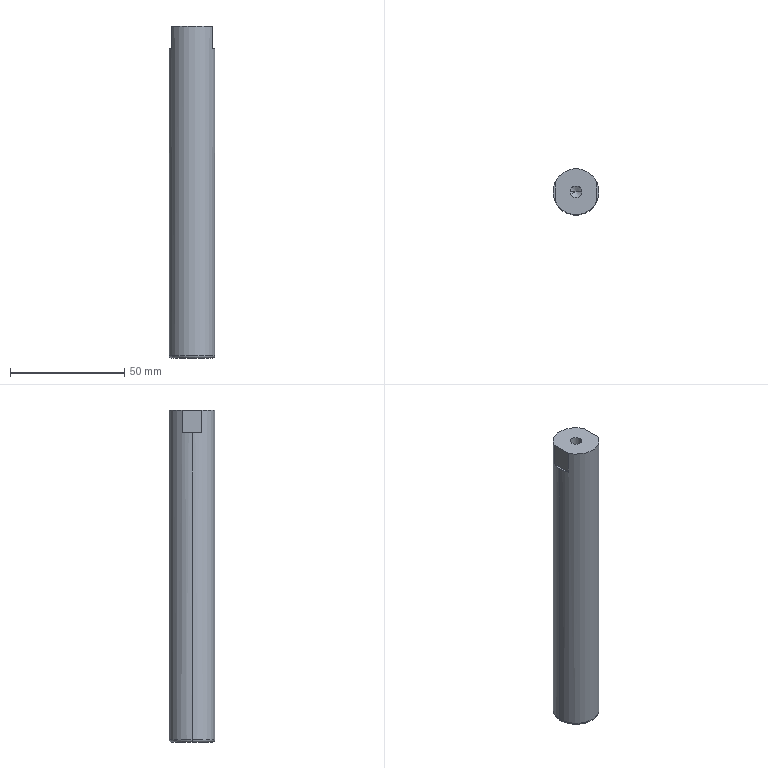Part | STEP file | 1 solid | 14 faces | box 20 x 20 x 145 mm | volume 45098 mm3 | plane 6 | cylinder 4 | torus 2 | cone 2 | commonest cylinder face diameters 5 x2 20 x2
STEP:
#1=CARTESIAN_POINT('',(0.,0.,0.));
#2=DIRECTION('',(0.,0.,1.));
#3=DIRECTION('',(1.,0.,0.));
#4=AXIS2_PLACEMENT_3D('',#1,#2,#3);
#5=CARTESIAN_POINT('',(-9.,0.,-72.5));
#6=VERTEX_POINT('',#5);
#7=CARTESIAN_POINT('',(9.,0.,-72.5));
#8=VERTEX_POINT('',#7);
#9=CARTESIAN_POINT('',(0.,0.,-72.5));
#10=DIRECTION('',(0.,0.,-1.));
#11=DIRECTION('',(1.,0.,0.));
#12=AXIS2_PLACEMENT_3D('',#9,#10,#11);
#13=CIRCLE('',#12,9.);
#14=CARTESIAN_POINT('',(0.,0.,-71.5));
#15=DIRECTION('',(0.,0.,1.));
#16=DIRECTION('',(1.,0.,0.));
#17=AXIS2_PLACEMENT_3D('',#14,#15,#16);
#18=TOROIDAL_SURFACE('',#17,9.,1.);
#19=CARTESIAN_POINT('',(6.283,4.712));
#20=DIRECTION('',(-1.,0.));
#21=VECTOR('',#20,1.);
#22=LINE('',#19,#21);
#23=(GEOMETRIC_REPRESENTATION_CONTEXT(2)PARAMETRIC_REPRESENTATION_CONTEXT()REPRESENTATION_CONTEXT('',''));
#24=DEFINITIONAL_REPRESENTATION('',(#22),#23);
#25=PCURVE('',#18,#24);
#26=CARTESIAN_POINT('',(0.,0.,-72.5));
#27=DIRECTION('',(0.,0.,1.));
#28=DIRECTION('',(1.,0.,0.));
#29=AXIS2_PLACEMENT_3D('',#26,#27,#28);
#30=PLANE('',#29);
#31=CARTESIAN_POINT('',(9.,0.));
#32=CARTESIAN_POINT('',(9.,-15.588));
#33=CARTESIAN_POINT('',(-4.5,-7.794));
#34=CARTESIAN_POINT('',(-18.,0.));
#35=CARTESIAN_POINT('',(-4.5,7.794));
#36=CARTESIAN_POINT('',(9.,15.588));
#37=CARTESIAN_POINT('',(9.,0.));
#38=(BOUNDED_CURVE()B_SPLINE_CURVE(2,(#31,#32,#33,#34,#35,#36,#37),.UNSPECIFIED.,.T.,.F.)B_SPLINE_CURVE_WITH_KNOTS((1,2,2,2,2,1),(-2.094,0.,2.094,4.189,6.283,8.378),.UNSPECIFIED.)CURVE()GEOMETRIC_REPRESENTATION_ITEM()RATIONAL_B_SPLINE_CURVE((1.,0.5,1.,0.5,1.,0.5,1.))REPRESENTATION_ITEM(''));
#39=(GEOMETRIC_REPRESENTATION_CONTEXT(2)PARAMETRIC_REPRESENTATION_CONTEXT()REPRESENTATION_CONTEXT('',''));
#40=DEFINITIONAL_REPRESENTATION('',(#38),#39);
#41=PCURVE('',#30,#40);
#42=SURFACE_CURVE('',#13,(#25,#41),.PCURVE_S1.);
#43=EDGE_CURVE('',#6,#8,#42,.T.);
#44=ORIENTED_EDGE('',*,*,#43,.F.);
#45=CARTESIAN_POINT('',(-10.,0.,-71.5));
#46=VERTEX_POINT('',#45);
#47=CARTESIAN_POINT('',(-9.,0.,-71.5));
#48=DIRECTION('',(0.,1.,0.));
#49=DIRECTION('',(-1.,0.,0.));
#50=AXIS2_PLACEMENT_3D('',#47,#48,#49);
#51=CIRCLE('',#50,1.);
#52=CARTESIAN_POINT('',(3.142,0.));
#53=DIRECTION('',(0.,1.));
#54=VECTOR('',#53,1.);
#55=LINE('',#52,#54);
#56=(GEOMETRIC_REPRESENTATION_CONTEXT(2)PARAMETRIC_REPRESENTATION_CONTEXT()REPRESENTATION_CONTEXT('',''));
#57=DEFINITIONAL_REPRESENTATION('',(#55),#56);
#58=PCURVE('',#18,#57);
#59=CARTESIAN_POINT('',(0.,0.,-71.5));
#60=DIRECTION('',(0.,0.,1.));
#61=DIRECTION('',(1.,0.,0.));
#62=AXIS2_PLACEMENT_3D('',#59,#60,#61);
#63=TOROIDAL_SURFACE('',#62,9.,1.);
#64=CARTESIAN_POINT('',(3.142,0.));
#65=DIRECTION('',(0.,1.));
#66=VECTOR('',#65,1.);
#67=LINE('',#64,#66);
#68=(GEOMETRIC_REPRESENTATION_CONTEXT(2)PARAMETRIC_REPRESENTATION_CONTEXT()REPRESENTATION_CONTEXT('',''));
#69=DEFINITIONAL_REPRESENTATION('',(#67),#68);
#70=PCURVE('',#63,#69);
#71=SURFACE_CURVE('',#51,(#58,#70),.PCURVE_S1.);
#72=EDGE_CURVE('',#6,#46,#71,.T.);
#73=ORIENTED_EDGE('',*,*,#72,.T.);
#74=CARTESIAN_POINT('',(10.,0.,-71.5));
#75=VERTEX_POINT('',#74);
#76=CARTESIAN_POINT('',(0.,0.,-71.5));
#77=DIRECTION('',(0.,0.,1.));
#78=DIRECTION('',(1.,0.,0.));
#79=AXIS2_PLACEMENT_3D('',#76,#77,#78);
#80=CIRCLE('',#79,10.);
#81=CARTESIAN_POINT('',(0.,6.283));
#82=DIRECTION('',(1.,0.));
#83=VECTOR('',#82,1.);
#84=LINE('',#81,#83);
#85=(GEOMETRIC_REPRESENTATION_CONTEXT(2)PARAMETRIC_REPRESENTATION_CONTEXT()REPRESENTATION_CONTEXT('',''));
#86=DEFINITIONAL_REPRESENTATION('',(#84),#85);
#87=PCURVE('',#18,#86);
#88=CARTESIAN_POINT('',(0.,0.,72.5));
#89=DIRECTION('',(0.,0.,-1.));
#90=DIRECTION('',(-1.,0.,0.));
#91=AXIS2_PLACEMENT_3D('',#88,#89,#90);
#92=CYLINDRICAL_SURFACE('',#91,10.);
#93=CARTESIAN_POINT('',(3.142,144.));
#94=DIRECTION('',(-1.,0.));
#95=VECTOR('',#94,1.);
#96=LINE('',#93,#95);
#97=(GEOMETRIC_REPRESENTATION_CONTEXT(2)PARAMETRIC_REPRESENTATION_CONTEXT()REPRESENTATION_CONTEXT('',''));
#98=DEFINITIONAL_REPRESENTATION('',(#96),#97);
#99=PCURVE('',#92,#98);
#100=SURFACE_CURVE('',#80,(#87,#99),.PCURVE_S1.);
#101=EDGE_CURVE('',#75,#46,#100,.T.);
#102=ORIENTED_EDGE('',*,*,#101,.F.);
#103=CARTESIAN_POINT('',(9.,0.,-71.5));
#104=DIRECTION('',(0.,-1.,0.));
#105=DIRECTION('',(0.,0.,-1.));
#106=AXIS2_PLACEMENT_3D('',#103,#104,#105);
#107=CIRCLE('',#106,1.);
#108=CARTESIAN_POINT('',(0.,4.712));
#109=DIRECTION('',(0.,1.));
#110=VECTOR('',#109,1.);
#111=LINE('',#108,#110);
#112=(GEOMETRIC_REPRESENTATION_CONTEXT(2)PARAMETRIC_REPRESENTATION_CONTEXT()REPRESENTATION_CONTEXT('',''));
#113=DEFINITIONAL_REPRESENTATION('',(#111),#112);
#114=PCURVE('',#18,#113);
#115=CARTESIAN_POINT('',(6.283,4.712));
#116=DIRECTION('',(0.,1.));
#117=VECTOR('',#116,1.);
#118=LINE('',#115,#117);
#119=(GEOMETRIC_REPRESENTATION_CONTEXT(2)PARAMETRIC_REPRESENTATION_CONTEXT()REPRESENTATION_CONTEXT('',''));
#120=DEFINITIONAL_REPRESENTATION('',(#118),#119);
#121=PCURVE('',#63,#120);
#122=SURFACE_CURVE('',#107,(#114,#121),.PCURVE_S1.);
#123=EDGE_CURVE('',#8,#75,#122,.T.);
#124=ORIENTED_EDGE('',*,*,#123,.F.);
#125=EDGE_LOOP('',(#44,#73,#102,#124));
#126=FACE_BOUND('',#125,.T.);
#127=ADVANCED_FACE('',(#126),#18,.T.);
#128=CARTESIAN_POINT('',(2.5,0.,56.5));
#129=VERTEX_POINT('',#128);
#130=CARTESIAN_POINT('',(2.5,0.,72.5));
#131=VERTEX_POINT('',#130);
#132=CARTESIAN_POINT('',(2.5,0.,72.5));
#133=DIRECTION('',(0.,0.,1.));
#134=VECTOR('',#133,1.);
#135=LINE('',#132,#134);
#136=CARTESIAN_POINT('',(0.,0.,72.5));
#137=DIRECTION('',(0.,0.,1.));
#138=DIRECTION('',(1.,0.,0.));
#139=AXIS2_PLACEMENT_3D('',#136,#137,#138);
#140=CYLINDRICAL_SURFACE('',#139,2.5);
#141=CARTESIAN_POINT('',(6.283,0.));
#142=DIRECTION('',(0.,1.));
#143=VECTOR('',#142,1.);
#144=LINE('',#141,#143);
#145=(GEOMETRIC_REPRESENTATION_CONTEXT(2)PARAMETRIC_REPRESENTATION_CONTEXT()REPRESENTATION_CONTEXT('',''));
#146=DEFINITIONAL_REPRESENTATION('',(#144),#145);
#147=PCURVE('',#140,#146);
#148=CARTESIAN_POINT('',(0.,0.,72.5));
#149=DIRECTION('',(0.,0.,1.));
#150=DIRECTION('',(1.,0.,0.));
#151=AXIS2_PLACEMENT_3D('',#148,#149,#150);
#152=CYLINDRICAL_SURFACE('',#151,2.5);
#153=CARTESIAN_POINT('',(0.,0.));
#154=DIRECTION('',(0.,1.));
#155=VECTOR('',#154,1.);
#156=LINE('',#153,#155);
#157=(GEOMETRIC_REPRESENTATION_CONTEXT(2)PARAMETRIC_REPRESENTATION_CONTEXT()REPRESENTATION_CONTEXT('',''));
#158=DEFINITIONAL_REPRESENTATION('',(#156),#157);
#159=PCURVE('',#152,#158);
#160=SURFACE_CURVE('',#135,(#147,#159),.PCURVE_S1.);
#161=EDGE_CURVE('',#129,#131,#160,.T.);
#162=ORIENTED_EDGE('',*,*,#161,.T.);
#163=CARTESIAN_POINT('',(-2.5,0.,72.5));
#164=VERTEX_POINT('',#163);
#165=CARTESIAN_POINT('',(0.,0.,72.5));
#166=DIRECTION('',(0.,0.,1.));
#167=DIRECTION('',(1.,0.,0.));
#168=AXIS2_PLACEMENT_3D('',#165,#166,#167);
#169=CIRCLE('',#168,2.5);
#170=CARTESIAN_POINT('',(0.,0.));
#171=DIRECTION('',(1.,0.));
#172=VECTOR('',#171,1.);
#173=LINE('',#170,#172);
#174=(GEOMETRIC_REPRESENTATION_CONTEXT(2)PARAMETRIC_REPRESENTATION_CONTEXT()REPRESENTATION_CONTEXT('',''));
#175=DEFINITIONAL_REPRESENTATION('',(#173),#174);
#176=PCURVE('',#140,#175);
#177=CARTESIAN_POINT('',(0.,0.,72.5));
#178=DIRECTION('',(0.,0.,1.));
#179=DIRECTION('',(1.,0.,0.));
#180=AXIS2_PLACEMENT_3D('',#177,#178,#179);
#181=PLANE('',#180);
#182=CARTESIAN_POINT('',(0.,0.));
#183=DIRECTION('',(1.,0.));
#184=AXIS2_PLACEMENT_2D('',#182,#183);
#185=CIRCLE('',#184,2.5);
#186=(GEOMETRIC_REPRESENTATION_CONTEXT(2)PARAMETRIC_REPRESENTATION_CONTEXT()REPRESENTATION_CONTEXT('',''));
#187=DEFINITIONAL_REPRESENTATION('',(#185),#186);
#188=PCURVE('',#181,#187);
#189=SURFACE_CURVE('',#169,(#176,#188),.PCURVE_S1.);
#190=EDGE_CURVE('',#164,#131,#189,.T.);
#191=ORIENTED_EDGE('',*,*,#190,.F.);
#192=CARTESIAN_POINT('',(-2.5,0.,56.5));
#193=VERTEX_POINT('',#192);
#194=CARTESIAN_POINT('',(-2.5,0.,72.5));
#195=DIRECTION('',(0.,0.,1.));
#196=VECTOR('',#195,1.);
#197=LINE('',#194,#196);
#198=CARTESIAN_POINT('',(3.142,0.));
#199=DIRECTION('',(0.,1.));
#200=VECTOR('',#199,1.);
#201=LINE('',#198,#200);
#202=(GEOMETRIC_REPRESENTATION_CONTEXT(2)PARAMETRIC_REPRESENTATION_CONTEXT()REPRESENTATION_CONTEXT('',''));
#203=DEFINITIONAL_REPRESENTATION('',(#201),#202);
#204=PCURVE('',#140,#203);
#205=CARTESIAN_POINT('',(3.142,0.));
#206=DIRECTION('',(0.,1.));
#207=VECTOR('',#206,1.);
#208=LINE('',#205,#207);
#209=(GEOMETRIC_REPRESENTATION_CONTEXT(2)PARAMETRIC_REPRESENTATION_CONTEXT()REPRESENTATION_CONTEXT('',''));
#210=DEFINITIONAL_REPRESENTATION('',(#208),#209);
#211=PCURVE('',#152,#210);
#212=SURFACE_CURVE('',#197,(#204,#211),.PCURVE_S1.);
#213=EDGE_CURVE('',#193,#164,#212,.T.);
#214=ORIENTED_EDGE('',*,*,#213,.F.);
#215=CARTESIAN_POINT('',(0.,0.,56.5));
#216=DIRECTION('',(0.,0.,1.));
#217=DIRECTION('',(1.,0.,0.));
#218=AXIS2_PLACEMENT_3D('',#215,#216,#217);
#219=CIRCLE('',#218,2.5);
#220=CARTESIAN_POINT('',(0.,-16.));
#221=DIRECTION('',(1.,0.));
#222=VECTOR('',#221,1.);
#223=LINE('',#220,#222);
#224=(GEOMETRIC_REPRESENTATION_CONTEXT(2)PARAMETRIC_REPRESENTATION_CONTEXT()REPRESENTATION_CONTEXT('',''));
#225=DEFINITIONAL_REPRESENTATION('',(#223),#224);
#226=PCURVE('',#140,#225);
#227=CARTESIAN_POINT('',(0.,0.,56.5));
#228=DIRECTION('',(0.,0.,1.));
#229=DIRECTION('',(1.,0.,0.));
#230=AXIS2_PLACEMENT_3D('',#227,#228,#229);
#231=CONICAL_SURFACE('',#230,2.5,1.03);
#232=CARTESIAN_POINT('',(0.,0.));
#233=DIRECTION('',(1.,0.));
#234=VECTOR('',#233,1.);
#235=LINE('',#232,#234);
#236=(GEOMETRIC_REPRESENTATION_CONTEXT(2)PARAMETRIC_REPRESENTATION_CONTEXT()REPRESENTATION_CONTEXT('',''));
#237=DEFINITIONAL_REPRESENTATION('',(#235),#236);
#238=PCURVE('',#231,#237);
#239=SURFACE_CURVE('',#219,(#226,#238),.PCURVE_S1.);
#240=EDGE_CURVE('',#193,#129,#239,.T.);
#241=ORIENTED_EDGE('',*,*,#240,.T.);
#242=EDGE_LOOP('',(#162,#191,#214,#241));
#243=FACE_BOUND('',#242,.F.);
#244=ADVANCED_FACE('',(#243),#140,.F.);
#245=ORIENTED_EDGE('',*,*,#240,.F.);
#246=CARTESIAN_POINT('',(0.,0.,54.998));
#247=VERTEX_POINT('',#246);
#248=CARTESIAN_POINT('',(-2.5,0.,56.5));
#249=DIRECTION('',(-0.8572,0.,0.515));
#250=VECTOR('',#249,1.);
#251=LINE('',#248,#250);
#252=CARTESIAN_POINT('',(3.142,0.));
#253=DIRECTION('',(0.,1.));
#254=VECTOR('',#253,1.);
#255=LINE('',#252,#254);
#256=(GEOMETRIC_REPRESENTATION_CONTEXT(2)PARAMETRIC_REPRESENTATION_CONTEXT()REPRESENTATION_CONTEXT('',''));
#257=DEFINITIONAL_REPRESENTATION('',(#255),#256);
#258=PCURVE('',#231,#257);
#259=CARTESIAN_POINT('',(0.,0.,56.5));
#260=DIRECTION('',(0.,0.,1.));
#261=DIRECTION('',(1.,0.,0.));
#262=AXIS2_PLACEMENT_3D('',#259,#260,#261);
#263=CONICAL_SURFACE('',#262,2.5,1.03);
#264=CARTESIAN_POINT('',(3.142,0.));
#265=DIRECTION('',(0.,1.));
#266=VECTOR('',#265,1.);
#267=LINE('',#264,#266);
#268=(GEOMETRIC_REPRESENTATION_CONTEXT(2)PARAMETRIC_REPRESENTATION_CONTEXT()REPRESENTATION_CONTEXT('',''));
#269=DEFINITIONAL_REPRESENTATION('',(#267),#268);
#270=PCURVE('',#263,#269);
#271=SURFACE_CURVE('',#251,(#258,#270),.PCURVE_S1.);
#272=EDGE_CURVE('',#247,#193,#271,.T.);
#273=ORIENTED_EDGE('',*,*,#272,.F.);
#274=CARTESIAN_POINT('',(2.5,0.,56.5));
#275=DIRECTION('',(0.8572,0.,0.515));
#276=VECTOR('',#275,1.);
#277=LINE('',#274,#276);
#278=CARTESIAN_POINT('',(6.283,0.));
#279=DIRECTION('',(0.,1.));
#280=VECTOR('',#279,1.);
#281=LINE('',#278,#280);
#282=(GEOMETRIC_REPRESENTATION_CONTEXT(2)PARAMETRIC_REPRESENTATION_CONTEXT()REPRESENTATION_CONTEXT('',''));
#283=DEFINITIONAL_REPRESENTATION('',(#281),#282);
#284=PCURVE('',#231,#283);
#285=CARTESIAN_POINT('',(0.,0.));
#286=DIRECTION('',(0.,1.));
#287=VECTOR('',#286,1.);
#288=LINE('',#285,#287);
#289=(GEOMETRIC_REPRESENTATION_CONTEXT(2)PARAMETRIC_REPRESENTATION_CONTEXT()REPRESENTATION_CONTEXT('',''));
#290=DEFINITIONAL_REPRESENTATION('',(#288),#289);
#291=PCURVE('',#263,#290);
#292=SURFACE_CURVE('',#277,(#284,#291),.PCURVE_S1.);
#293=EDGE_CURVE('',#247,#129,#292,.T.);
#294=ORIENTED_EDGE('',*,*,#293,.T.);
#295=EDGE_LOOP('',(#245,#273,#294));
#296=FACE_BOUND('',#295,.F.);
#297=ADVANCED_FACE('',(#296),#231,.F.);
#298=CARTESIAN_POINT('',(10.,0.,62.5));
#299=VERTEX_POINT('',#298);
#300=CARTESIAN_POINT('',(9.,4.359,62.5));
#301=VERTEX_POINT('',#300);
#302=CARTESIAN_POINT('',(0.,0.,62.5));
#303=DIRECTION('',(0.,0.,1.));
#304=DIRECTION('',(1.,0.,0.));
#305=AXIS2_PLACEMENT_3D('',#302,#303,#304);
#306=CIRCLE('',#305,10.);
#307=CARTESIAN_POINT('',(3.142,10.));
#308=DIRECTION('',(-1.,0.));
#309=VECTOR('',#308,1.);
#310=LINE('',#307,#309);
#311=(GEOMETRIC_REPRESENTATION_CONTEXT(2)PARAMETRIC_REPRESENTATION_CONTEXT()REPRESENTATION_CONTEXT('',''));
#312=DEFINITIONAL_REPRESENTATION('',(#310),#311);
#313=PCURVE('',#92,#312);
#314=CARTESIAN_POINT('',(0.,0.,62.5));
#315=DIRECTION('',(0.,0.,1.));
#316=DIRECTION('',(1.,0.,0.));
#317=AXIS2_PLACEMENT_3D('',#314,#315,#316);
#318=PLANE('',#317);
#319=CARTESIAN_POINT('',(0.,0.));
#320=DIRECTION('',(1.,0.));
#321=AXIS2_PLACEMENT_2D('',#319,#320);
#322=CIRCLE('',#321,10.);
#323=(GEOMETRIC_REPRESENTATION_CONTEXT(2)PARAMETRIC_REPRESENTATION_CONTEXT()REPRESENTATION_CONTEXT('',''));
#324=DEFINITIONAL_REPRESENTATION('',(#322),#323);
#325=PCURVE('',#318,#324);
#326=SURFACE_CURVE('',#306,(#313,#325),.PCURVE_S1.);
#327=EDGE_CURVE('',#299,#301,#326,.T.);
#328=ORIENTED_EDGE('',*,*,#327,.F.);
#329=CARTESIAN_POINT('',(10.,0.,72.5));
#330=DIRECTION('',(0.,0.,-1.));
#331=VECTOR('',#330,1.);
#332=LINE('',#329,#331);
#333=CARTESIAN_POINT('',(3.142,0.));
#334=DIRECTION('',(0.,1.));
#335=VECTOR('',#334,1.);
#336=LINE('',#333,#335);
#337=(GEOMETRIC_REPRESENTATION_CONTEXT(2)PARAMETRIC_REPRESENTATION_CONTEXT()REPRESENTATION_CONTEXT('',''));
#338=DEFINITIONAL_REPRESENTATION('',(#336),#337);
#339=PCURVE('',#92,#338);
#340=CARTESIAN_POINT('',(0.,0.,72.5));
#341=DIRECTION('',(0.,0.,-1.));
#342=DIRECTION('',(-1.,0.,0.));
#343=AXIS2_PLACEMENT_3D('',#340,#341,#342);
#344=CYLINDRICAL_SURFACE('',#343,10.);
#345=CARTESIAN_POINT('',(3.142,0.));
#346=DIRECTION('',(0.,1.));
#347=VECTOR('',#346,1.);
#348=LINE('',#345,#347);
#349=(GEOMETRIC_REPRESENTATION_CONTEXT(2)PARAMETRIC_REPRESENTATION_CONTEXT()REPRESENTATION_CONTEXT('',''));
#350=DEFINITIONAL_REPRESENTATION('',(#348),#349);
#351=PCURVE('',#344,#350);
#352=SURFACE_CURVE('',#332,(#339,#351),.PCURVE_S1.);
#353=EDGE_CURVE('',#299,#75,#352,.T.);
#354=ORIENTED_EDGE('',*,*,#353,.T.);
#355=ORIENTED_EDGE('',*,*,#101,.T.);
#356=CARTESIAN_POINT('',(-10.,0.,62.5));
#357=VERTEX_POINT('',#356);
#358=CARTESIAN_POINT('',(-10.,0.,72.5));
#359=DIRECTION('',(0.,0.,-1.));
#360=VECTOR('',#359,1.);
#361=LINE('',#358,#360);
#362=CARTESIAN_POINT('',(0.,0.));
#363=DIRECTION('',(0.,1.));
#364=VECTOR('',#363,1.);
#365=LINE('',#362,#364);
#366=(GEOMETRIC_REPRESENTATION_CONTEXT(2)PARAMETRIC_REPRESENTATION_CONTEXT()REPRESENTATION_CONTEXT('',''));
#367=DEFINITIONAL_REPRESENTATION('',(#365),#366);
#368=PCURVE('',#92,#367);
#369=CARTESIAN_POINT('',(6.283,0.));
#370=DIRECTION('',(0.,1.));
#371=VECTOR('',#370,1.);
#372=LINE('',#369,#371);
#373=(GEOMETRIC_REPRESENTATION_CONTEXT(2)PARAMETRIC_REPRESENTATION_CONTEXT()REPRESENTATION_CONTEXT('',''));
#374=DEFINITIONAL_REPRESENTATION('',(#372),#373);
#375=PCURVE('',#344,#374);
#376=SURFACE_CURVE('',#361,(#368,#375),.PCURVE_S1.);
#377=EDGE_CURVE('',#357,#46,#376,.T.);
#378=ORIENTED_EDGE('',*,*,#377,.F.);
#379=CARTESIAN_POINT('',(-9.,4.359,62.5));
#380=VERTEX_POINT('',#379);
#381=CARTESIAN_POINT('',(0.,0.,62.5));
#382=DIRECTION('',(0.,0.,1.));
#383=DIRECTION('',(1.,0.,0.));
#384=AXIS2_PLACEMENT_3D('',#381,#382,#383);
#385=CIRCLE('',#384,10.);
#386=CARTESIAN_POINT('',(3.142,10.));
#387=DIRECTION('',(-1.,0.));
#388=VECTOR('',#387,1.);
#389=LINE('',#386,#388);
#390=(GEOMETRIC_REPRESENTATION_CONTEXT(2)PARAMETRIC_REPRESENTATION_CONTEXT()REPRESENTATION_CONTEXT('',''));
#391=DEFINITIONAL_REPRESENTATION('',(#389),#390);
#392=PCURVE('',#92,#391);
#393=CARTESIAN_POINT('',(0.,0.,62.5));
#394=DIRECTION('',(0.,0.,1.));
#395=DIRECTION('',(1.,0.,0.));
#396=AXIS2_PLACEMENT_3D('',#393,#394,#395);
#397=PLANE('',#396);
#398=CARTESIAN_POINT('',(0.,0.));
#399=DIRECTION('',(1.,0.));
#400=AXIS2_PLACEMENT_2D('',#398,#399);
#401=CIRCLE('',#400,10.);
#402=(GEOMETRIC_REPRESENTATION_CONTEXT(2)PARAMETRIC_REPRESENTATION_CONTEXT()REPRESENTATION_CONTEXT('',''));
#403=DEFINITIONAL_REPRESENTATION('',(#401),#402);
#404=PCURVE('',#397,#403);
#405=SURFACE_CURVE('',#385,(#392,#404),.PCURVE_S1.);
#406=EDGE_CURVE('',#380,#357,#405,.T.);
#407=ORIENTED_EDGE('',*,*,#406,.F.);
#408=CARTESIAN_POINT('',(-9.,4.359,72.5));
#409=VERTEX_POINT('',#408);
#410=CARTESIAN_POINT('',(-9.,4.359,72.5));
#411=DIRECTION('',(0.,0.,-1.));
#412=VECTOR('',#411,1.);
#413=LINE('',#410,#412);
#414=CARTESIAN_POINT('',(0.451,0.));
#415=DIRECTION('',(0.,1.));
#416=VECTOR('',#415,1.);
#417=LINE('',#414,#416);
#418=(GEOMETRIC_REPRESENTATION_CONTEXT(2)PARAMETRIC_REPRESENTATION_CONTEXT()REPRESENTATION_CONTEXT('',''));
#419=DEFINITIONAL_REPRESENTATION('',(#417),#418);
#420=PCURVE('',#92,#419);
#421=CARTESIAN_POINT('',(-9.,-11.827,62.5));
#422=DIRECTION('',(-1.,0.,0.));
#423=DIRECTION('',(0.,0.,1.));
#424=AXIS2_PLACEMENT_3D('',#421,#422,#423);
#425=PLANE('',#424);
#426=CARTESIAN_POINT('',(10.,16.185));
#427=DIRECTION('',(-1.,0.));
#428=VECTOR('',#427,1.);
#429=LINE('',#426,#428);
#430=(GEOMETRIC_REPRESENTATION_CONTEXT(2)PARAMETRIC_REPRESENTATION_CONTEXT()REPRESENTATION_CONTEXT('',''));
#431=DEFINITIONAL_REPRESENTATION('',(#429),#430);
#432=PCURVE('',#425,#431);
#433=SURFACE_CURVE('',#413,(#420,#432),.PCURVE_S1.);
#434=EDGE_CURVE('',#409,#380,#433,.T.);
#435=ORIENTED_EDGE('',*,*,#434,.F.);
#436=CARTESIAN_POINT('',(9.,4.359,72.5));
#437=VERTEX_POINT('',#436);
#438=CARTESIAN_POINT('',(0.,0.,72.5));
#439=DIRECTION('',(0.,0.,1.));
#440=DIRECTION('',(1.,0.,0.));
#441=AXIS2_PLACEMENT_3D('',#438,#439,#440);
#442=CIRCLE('',#441,10.);
#443=CARTESIAN_POINT('',(3.142,0.));
#444=DIRECTION('',(-1.,0.));
#445=VECTOR('',#444,1.);
#446=LINE('',#443,#445);
#447=(GEOMETRIC_REPRESENTATION_CONTEXT(2)PARAMETRIC_REPRESENTATION_CONTEXT()REPRESENTATION_CONTEXT('',''));
#448=DEFINITIONAL_REPRESENTATION('',(#446),#447);
#449=PCURVE('',#92,#448);
#450=CARTESIAN_POINT('',(0.,0.));
#451=DIRECTION('',(1.,0.));
#452=AXIS2_PLACEMENT_2D('',#450,#451);
#453=CIRCLE('',#452,10.);
#454=(GEOMETRIC_REPRESENTATION_CONTEXT(2)PARAMETRIC_REPRESENTATION_CONTEXT()REPRESENTATION_CONTEXT('',''));
#455=DEFINITIONAL_REPRESENTATION('',(#453),#454);
#456=PCURVE('',#181,#455);
#457=SURFACE_CURVE('',#442,(#449,#456),.PCURVE_S1.);
#458=EDGE_CURVE('',#437,#409,#457,.T.);
#459=ORIENTED_EDGE('',*,*,#458,.F.);
#460=CARTESIAN_POINT('',(9.,4.359,72.5));
#461=DIRECTION('',(0.,0.,1.));
#462=VECTOR('',#461,1.);
#463=LINE('',#460,#462);
#464=CARTESIAN_POINT('',(2.691,0.));
#465=DIRECTION('',(0.,-1.));
#466=VECTOR('',#465,1.);
#467=LINE('',#464,#466);
#468=(GEOMETRIC_REPRESENTATION_CONTEXT(2)PARAMETRIC_REPRESENTATION_CONTEXT()REPRESENTATION_CONTEXT('',''));
#469=DEFINITIONAL_REPRESENTATION('',(#467),#468);
#470=PCURVE('',#92,#469);
#471=CARTESIAN_POINT('',(9.,-11.827,62.5));
#472=DIRECTION('',(1.,0.,0.));
#473=DIRECTION('',(0.,0.,-1.));
#474=AXIS2_PLACEMENT_3D('',#471,#472,#473);
#475=PLANE('',#474);
#476=CARTESIAN_POINT('',(-10.,16.185));
#477=DIRECTION('',(-1.,0.));
#478=VECTOR('',#477,1.);
#479=LINE('',#476,#478);
#480=(GEOMETRIC_REPRESENTATION_CONTEXT(2)PARAMETRIC_REPRESENTATION_CONTEXT()REPRESENTATION_CONTEXT('',''));
#481=DEFINITIONAL_REPRESENTATION('',(#479),#480);
#482=PCURVE('',#475,#481);
#483=SURFACE_CURVE('',#463,(#470,#482),.PCURVE_S1.);
#484=EDGE_CURVE('',#301,#437,#483,.T.);
#485=ORIENTED_EDGE('',*,*,#484,.F.);
#486=EDGE_LOOP('',(#328,#354,#355,#378,#407,#435,#459,#485));
#487=FACE_BOUND('',#486,.T.);
#488=ADVANCED_FACE('',(#487),#92,.T.);
#489=ORIENTED_EDGE('',*,*,#353,.F.);
#490=CARTESIAN_POINT('',(9.,-4.359,62.5));
#491=VERTEX_POINT('',#490);
#492=CARTESIAN_POINT('',(0.,0.,62.5));
#493=DIRECTION('',(0.,0.,1.));
#494=DIRECTION('',(1.,0.,0.));
#495=AXIS2_PLACEMENT_3D('',#492,#493,#494);
#496=CIRCLE('',#495,10.);
#497=CARTESIAN_POINT('',(9.425,10.));
#498=DIRECTION('',(-1.,0.));
#499=VECTOR('',#498,1.);
#500=LINE('',#497,#499);
#501=(GEOMETRIC_REPRESENTATION_CONTEXT(2)PARAMETRIC_REPRESENTATION_CONTEXT()REPRESENTATION_CONTEXT('',''));
#502=DEFINITIONAL_REPRESENTATION('',(#500),#501);
#503=PCURVE('',#344,#502);
#504=CARTESIAN_POINT('',(0.,0.));
#505=DIRECTION('',(1.,0.));
#506=AXIS2_PLACEMENT_2D('',#504,#505);
#507=CIRCLE('',#506,10.);
#508=(GEOMETRIC_REPRESENTATION_CONTEXT(2)PARAMETRIC_REPRESENTATION_CONTEXT()REPRESENTATION_CONTEXT('',''));
#509=DEFINITIONAL_REPRESENTATION('',(#507),#508);
#510=PCURVE('',#318,#509);
#511=SURFACE_CURVE('',#496,(#503,#510),.PCURVE_S1.);
#512=EDGE_CURVE('',#491,#299,#511,.T.);
#513=ORIENTED_EDGE('',*,*,#512,.F.);
#514=CARTESIAN_POINT('',(9.,-4.359,72.5));
#515=VERTEX_POINT('',#514);
#516=CARTESIAN_POINT('',(9.,-4.359,72.5));
#517=DIRECTION('',(0.,0.,-1.));
#518=VECTOR('',#517,1.);
#519=LINE('',#516,#518);
#520=CARTESIAN_POINT('',(3.593,0.));
#521=DIRECTION('',(0.,1.));
#522=VECTOR('',#521,1.);
#523=LINE('',#520,#522);
#524=(GEOMETRIC_REPRESENTATION_CONTEXT(2)PARAMETRIC_REPRESENTATION_CONTEXT()REPRESENTATION_CONTEXT('',''));
#525=DEFINITIONAL_REPRESENTATION('',(#523),#524);
#526=PCURVE('',#344,#525);
#527=CARTESIAN_POINT('',(-10.,7.468));
#528=DIRECTION('',(1.,0.));
#529=VECTOR('',#528,1.);
#530=LINE('',#527,#529);
#531=(GEOMETRIC_REPRESENTATION_CONTEXT(2)PARAMETRIC_REPRESENTATION_CONTEXT()REPRESENTATION_CONTEXT('',''));
#532=DEFINITIONAL_REPRESENTATION('',(#530),#531);
#533=PCURVE('',#475,#532);
#534=SURFACE_CURVE('',#519,(#526,#533),.PCURVE_S1.);
#535=EDGE_CURVE('',#515,#491,#534,.T.);
#536=ORIENTED_EDGE('',*,*,#535,.F.);
#537=CARTESIAN_POINT('',(-9.,-4.359,72.5));
#538=VERTEX_POINT('',#537);
#539=CARTESIAN_POINT('',(0.,0.,72.5));
#540=DIRECTION('',(0.,0.,1.));
#541=DIRECTION('',(1.,0.,0.));
#542=AXIS2_PLACEMENT_3D('',#539,#540,#541);
#543=CIRCLE('',#542,10.);
#544=CARTESIAN_POINT('',(9.425,0.));
#545=DIRECTION('',(-1.,0.));
#546=VECTOR('',#545,1.);
#547=LINE('',#544,#546);
#548=(GEOMETRIC_REPRESENTATION_CONTEXT(2)PARAMETRIC_REPRESENTATION_CONTEXT()REPRESENTATION_CONTEXT('',''));
#549=DEFINITIONAL_REPRESENTATION('',(#547),#548);
#550=PCURVE('',#344,#549);
#551=CARTESIAN_POINT('',(0.,0.));
#552=DIRECTION('',(1.,0.));
#553=AXIS2_PLACEMENT_2D('',#551,#552);
#554=CIRCLE('',#553,10.);
#555=(GEOMETRIC_REPRESENTATION_CONTEXT(2)PARAMETRIC_REPRESENTATION_CONTEXT()REPRESENTATION_CONTEXT('',''));
#556=DEFINITIONAL_REPRESENTATION('',(#554),#555);
#557=PCURVE('',#181,#556);
#558=SURFACE_CURVE('',#543,(#550,#557),.PCURVE_S1.);
#559=EDGE_CURVE('',#538,#515,#558,.T.);
#560=ORIENTED_EDGE('',*,*,#559,.F.);
#561=CARTESIAN_POINT('',(-9.,-4.359,62.5));
#562=VERTEX_POINT('',#561);
#563=CARTESIAN_POINT('',(-9.,-4.359,72.5));
#564=DIRECTION('',(0.,0.,1.));
#565=VECTOR('',#564,1.);
#566=LINE('',#563,#565);
#567=CARTESIAN_POINT('',(5.832,0.));
#568=DIRECTION('',(0.,-1.));
#569=VECTOR('',#568,1.);
#570=LINE('',#567,#569);
#571=(GEOMETRIC_REPRESENTATION_CONTEXT(2)PARAMETRIC_REPRESENTATION_CONTEXT()REPRESENTATION_CONTEXT('',''));
#572=DEFINITIONAL_REPRESENTATION('',(#570),#571);
#573=PCURVE('',#344,#572);
#574=CARTESIAN_POINT('',(10.,7.468));
#575=DIRECTION('',(1.,0.));
#576=VECTOR('',#575,1.);
#577=LINE('',#574,#576);
#578=(GEOMETRIC_REPRESENTATION_CONTEXT(2)PARAMETRIC_REPRESENTATION_CONTEXT()REPRESENTATION_CONTEXT('',''));
#579=DEFINITIONAL_REPRESENTATION('',(#577),#578);
#580=PCURVE('',#425,#579);
#581=SURFACE_CURVE('',#566,(#573,#580),.PCURVE_S1.);
#582=EDGE_CURVE('',#562,#538,#581,.T.);
#583=ORIENTED_EDGE('',*,*,#582,.F.);
#584=CARTESIAN_POINT('',(0.,0.,62.5));
#585=DIRECTION('',(0.,0.,1.));
#586=DIRECTION('',(1.,0.,0.));
#587=AXIS2_PLACEMENT_3D('',#584,#585,#586);
#588=CIRCLE('',#587,10.);
#589=CARTESIAN_POINT('',(9.425,10.));
#590=DIRECTION('',(-1.,0.));
#591=VECTOR('',#590,1.);
#592=LINE('',#589,#591);
#593=(GEOMETRIC_REPRESENTATION_CONTEXT(2)PARAMETRIC_REPRESENTATION_CONTEXT()REPRESENTATION_CONTEXT('',''));
#594=DEFINITIONAL_REPRESENTATION('',(#592),#593);
#595=PCURVE('',#344,#594);
#596=CARTESIAN_POINT('',(0.,0.));
#597=DIRECTION('',(1.,0.));
#598=AXIS2_PLACEMENT_2D('',#596,#597);
#599=CIRCLE('',#598,10.);
#600=(GEOMETRIC_REPRESENTATION_CONTEXT(2)PARAMETRIC_REPRESENTATION_CONTEXT()REPRESENTATION_CONTEXT('',''));
#601=DEFINITIONAL_REPRESENTATION('',(#599),#600);
#602=PCURVE('',#397,#601);
#603=SURFACE_CURVE('',#588,(#595,#602),.PCURVE_S1.);
#604=EDGE_CURVE('',#357,#562,#603,.T.);
#605=ORIENTED_EDGE('',*,*,#604,.F.);
#606=ORIENTED_EDGE('',*,*,#377,.T.);
#607=CARTESIAN_POINT('',(0.,0.,-71.5));
#608=DIRECTION('',(0.,0.,1.));
#609=DIRECTION('',(1.,0.,0.));
#610=AXIS2_PLACEMENT_3D('',#607,#608,#609);
#611=CIRCLE('',#610,10.);
#612=CARTESIAN_POINT('',(9.425,144.));
#613=DIRECTION('',(-1.,0.));
#614=VECTOR('',#613,1.);
#615=LINE('',#612,#614);
#616=(GEOMETRIC_REPRESENTATION_CONTEXT(2)PARAMETRIC_REPRESENTATION_CONTEXT()REPRESENTATION_CONTEXT('',''));
#617=DEFINITIONAL_REPRESENTATION('',(#615),#616);
#618=PCURVE('',#344,#617);
#619=CARTESIAN_POINT('',(0.,6.283));
#620=DIRECTION('',(1.,0.));
#621=VECTOR('',#620,1.);
#622=LINE('',#619,#621);
#623=(GEOMETRIC_REPRESENTATION_CONTEXT(2)PARAMETRIC_REPRESENTATION_CONTEXT()REPRESENTATION_CONTEXT('',''));
#624=DEFINITIONAL_REPRESENTATION('',(#622),#623);
#625=PCURVE('',#63,#624);
#626=SURFACE_CURVE('',#611,(#618,#625),.PCURVE_S1.);
#627=EDGE_CURVE('',#46,#75,#626,.T.);
#628=ORIENTED_EDGE('',*,*,#627,.T.);
#629=EDGE_LOOP('',(#489,#513,#536,#560,#583,#605,#606,#628));
#630=FACE_BOUND('',#629,.T.);
#631=ADVANCED_FACE('',(#630),#344,.T.);
#632=CARTESIAN_POINT('',(0.,0.,72.5));
#633=DIRECTION('',(0.,0.,1.));
#634=DIRECTION('',(1.,0.,0.));
#635=AXIS2_PLACEMENT_3D('',#632,#633,#634);
#636=CIRCLE('',#635,2.5);
#637=CARTESIAN_POINT('',(0.,0.));
#638=DIRECTION('',(1.,0.));
#639=AXIS2_PLACEMENT_2D('',#637,#638);
#640=CIRCLE('',#639,2.5);
#641=(GEOMETRIC_REPRESENTATION_CONTEXT(2)PARAMETRIC_REPRESENTATION_CONTEXT()REPRESENTATION_CONTEXT('',''));
#642=DEFINITIONAL_REPRESENTATION('',(#640),#641);
#643=PCURVE('',#181,#642);
#644=CARTESIAN_POINT('',(0.,0.));
#645=DIRECTION('',(1.,0.));
#646=VECTOR('',#645,1.);
#647=LINE('',#644,#646);
#648=(GEOMETRIC_REPRESENTATION_CONTEXT(2)PARAMETRIC_REPRESENTATION_CONTEXT()REPRESENTATION_CONTEXT('',''));
#649=DEFINITIONAL_REPRESENTATION('',(#647),#648);
#650=PCURVE('',#152,#649);
#651=SURFACE_CURVE('',#636,(#643,#650),.PCURVE_S1.);
#652=EDGE_CURVE('',#131,#164,#651,.T.);
#653=ORIENTED_EDGE('',*,*,#652,.F.);
#654=ORIENTED_EDGE('',*,*,#190,.F.);
#655=EDGE_LOOP('',(#653,#654));
#656=FACE_BOUND('',#655,.T.);
#657=ORIENTED_EDGE('',*,*,#559,.T.);
#658=CARTESIAN_POINT('',(9.,0.,72.5));
#659=DIRECTION('',(0.,1.,0.));
#660=VECTOR('',#659,1.);
#661=LINE('',#658,#660);
#662=CARTESIAN_POINT('',(9.,0.));
#663=DIRECTION('',(0.,1.));
#664=VECTOR('',#663,1.);
#665=LINE('',#662,#664);
#666=(GEOMETRIC_REPRESENTATION_CONTEXT(2)PARAMETRIC_REPRESENTATION_CONTEXT()REPRESENTATION_CONTEXT('',''));
#667=DEFINITIONAL_REPRESENTATION('',(#665),#666);
#668=PCURVE('',#181,#667);
#669=CARTESIAN_POINT('',(-10.,11.827));
#670=DIRECTION('',(0.,1.));
#671=VECTOR('',#670,1.);
#672=LINE('',#669,#671);
#673=(GEOMETRIC_REPRESENTATION_CONTEXT(2)PARAMETRIC_REPRESENTATION_CONTEXT()REPRESENTATION_CONTEXT('',''));
#674=DEFINITIONAL_REPRESENTATION('',(#672),#673);
#675=PCURVE('',#475,#674);
#676=SURFACE_CURVE('',#661,(#668,#675),.PCURVE_S1.);
#677=EDGE_CURVE('',#515,#437,#676,.T.);
#678=ORIENTED_EDGE('',*,*,#677,.T.);
#679=ORIENTED_EDGE('',*,*,#458,.T.);
#680=CARTESIAN_POINT('',(-9.,0.,72.5));
#681=DIRECTION('',(0.,-1.,0.));
#682=VECTOR('',#681,1.);
#683=LINE('',#680,#682);
#684=CARTESIAN_POINT('',(-9.,0.));
#685=DIRECTION('',(0.,-1.));
#686=VECTOR('',#685,1.);
#687=LINE('',#684,#686);
#688=(GEOMETRIC_REPRESENTATION_CONTEXT(2)PARAMETRIC_REPRESENTATION_CONTEXT()REPRESENTATION_CONTEXT('',''));
#689=DEFINITIONAL_REPRESENTATION('',(#687),#688);
#690=PCURVE('',#181,#689);
#691=CARTESIAN_POINT('',(10.,11.827));
#692=DIRECTION('',(0.,-1.));
#693=VECTOR('',#692,1.);
#694=LINE('',#691,#693);
#695=(GEOMETRIC_REPRESENTATION_CONTEXT(2)PARAMETRIC_REPRESENTATION_CONTEXT()REPRESENTATION_CONTEXT('',''));
#696=DEFINITIONAL_REPRESENTATION('',(#694),#695);
#697=PCURVE('',#425,#696);
#698=SURFACE_CURVE('',#683,(#690,#697),.PCURVE_S1.);
#699=EDGE_CURVE('',#409,#538,#698,.T.);
#700=ORIENTED_EDGE('',*,*,#699,.T.);
#701=EDGE_LOOP('',(#657,#678,#679,#700));
#702=FACE_BOUND('',#701,.T.);
#703=ADVANCED_FACE('',(#656,#702),#181,.T.);
#704=CARTESIAN_POINT('',(0.,0.,-72.5));
#705=DIRECTION('',(0.,0.,-1.));
#706=DIRECTION('',(1.,0.,0.));
#707=AXIS2_PLACEMENT_3D('',#704,#705,#706);
#708=CIRCLE('',#707,9.);
#709=CARTESIAN_POINT('',(9.,0.));
#710=CARTESIAN_POINT('',(9.,-15.588));
#711=CARTESIAN_POINT('',(-4.5,-7.794));
#712=CARTESIAN_POINT('',(-18.,0.));
#713=CARTESIAN_POINT('',(-4.5,7.794));
#714=CARTESIAN_POINT('',(9.,15.588));
#715=CARTESIAN_POINT('',(9.,0.));
#716=(BOUNDED_CURVE()B_SPLINE_CURVE(2,(#709,#710,#711,#712,#713,#714,#715),.UNSPECIFIED.,.T.,.F.)B_SPLINE_CURVE_WITH_KNOTS((1,2,2,2,2,1),(-2.094,0.,2.094,4.189,6.283,8.378),.UNSPECIFIED.)CURVE()GEOMETRIC_REPRESENTATION_ITEM()RATIONAL_B_SPLINE_CURVE((1.,0.5,1.,0.5,1.,0.5,1.))REPRESENTATION_ITEM(''));
#717=(GEOMETRIC_REPRESENTATION_CONTEXT(2)PARAMETRIC_REPRESENTATION_CONTEXT()REPRESENTATION_CONTEXT('',''));
#718=DEFINITIONAL_REPRESENTATION('',(#716),#717);
#719=PCURVE('',#30,#718);
#720=CARTESIAN_POINT('',(6.283,4.712));
#721=DIRECTION('',(-1.,0.));
#722=VECTOR('',#721,1.);
#723=LINE('',#720,#722);
#724=(GEOMETRIC_REPRESENTATION_CONTEXT(2)PARAMETRIC_REPRESENTATION_CONTEXT()REPRESENTATION_CONTEXT('',''));
#725=DEFINITIONAL_REPRESENTATION('',(#723),#724);
#726=PCURVE('',#63,#725);
#727=SURFACE_CURVE('',#708,(#719,#726),.PCURVE_S1.);
#728=EDGE_CURVE('',#8,#6,#727,.T.);
#729=ORIENTED_EDGE('',*,*,#728,.T.);
#730=ORIENTED_EDGE('',*,*,#43,.T.);
#731=EDGE_LOOP('',(#729,#730));
#732=FACE_BOUND('',#731,.T.);
#733=ADVANCED_FACE('',(#732),#30,.F.);
#734=CARTESIAN_POINT('',(0.,0.,56.5));
#735=DIRECTION('',(0.,0.,1.));
#736=DIRECTION('',(1.,0.,0.));
#737=AXIS2_PLACEMENT_3D('',#734,#735,#736);
#738=CIRCLE('',#737,2.5);
#739=CARTESIAN_POINT('',(0.,0.));
#740=DIRECTION('',(1.,0.));
#741=VECTOR('',#740,1.);
#742=LINE('',#739,#741);
#743=(GEOMETRIC_REPRESENTATION_CONTEXT(2)PARAMETRIC_REPRESENTATION_CONTEXT()REPRESENTATION_CONTEXT('',''));
#744=DEFINITIONAL_REPRESENTATION('',(#742),#743);
#745=PCURVE('',#263,#744);
#746=CARTESIAN_POINT('',(0.,-16.));
#747=DIRECTION('',(1.,0.));
#748=VECTOR('',#747,1.);
#749=LINE('',#746,#748);
#750=(GEOMETRIC_REPRESENTATION_CONTEXT(2)PARAMETRIC_REPRESENTATION_CONTEXT()REPRESENTATION_CONTEXT('',''));
#751=DEFINITIONAL_REPRESENTATION('',(#749),#750);
#752=PCURVE('',#152,#751);
#753=SURFACE_CURVE('',#738,(#745,#752),.PCURVE_S1.);
#754=EDGE_CURVE('',#129,#193,#753,.T.);
#755=ORIENTED_EDGE('',*,*,#754,.F.);
#756=ORIENTED_EDGE('',*,*,#293,.F.);
#757=ORIENTED_EDGE('',*,*,#272,.T.);
#758=EDGE_LOOP('',(#755,#756,#757));
#759=FACE_BOUND('',#758,.F.);
#760=ADVANCED_FACE('',(#759),#263,.F.);
#761=ORIENTED_EDGE('',*,*,#652,.F.);
#762=ORIENTED_EDGE('',*,*,#161,.F.);
#763=ORIENTED_EDGE('',*,*,#754,.T.);
#764=ORIENTED_EDGE('',*,*,#213,.T.);
#765=EDGE_LOOP('',(#761,#762,#763,#764));
#766=FACE_BOUND('',#765,.F.);
#767=ADVANCED_FACE('',(#766),#152,.F.);
#768=ORIENTED_EDGE('',*,*,#434,.T.);
#769=CARTESIAN_POINT('',(-9.,-11.827,62.5));
#770=DIRECTION('',(0.,-1.,0.));
#771=VECTOR('',#770,1.);
#772=LINE('',#769,#771);
#773=CARTESIAN_POINT('',(0.,0.));
#774=DIRECTION('',(0.,-1.));
#775=VECTOR('',#774,1.);
#776=LINE('',#773,#775);
#777=(GEOMETRIC_REPRESENTATION_CONTEXT(2)PARAMETRIC_REPRESENTATION_CONTEXT()REPRESENTATION_CONTEXT('',''));
#778=DEFINITIONAL_REPRESENTATION('',(#776),#777);
#779=PCURVE('',#425,#778);
#780=CARTESIAN_POINT('',(-9.,-11.827));
#781=DIRECTION('',(0.,-1.));
#782=VECTOR('',#781,1.);
#783=LINE('',#780,#782);
#784=(GEOMETRIC_REPRESENTATION_CONTEXT(2)PARAMETRIC_REPRESENTATION_CONTEXT()REPRESENTATION_CONTEXT('',''));
#785=DEFINITIONAL_REPRESENTATION('',(#783),#784);
#786=PCURVE('',#397,#785);
#787=SURFACE_CURVE('',#772,(#779,#786),.PCURVE_S1.);
#788=EDGE_CURVE('',#380,#562,#787,.T.);
#789=ORIENTED_EDGE('',*,*,#788,.T.);
#790=ORIENTED_EDGE('',*,*,#582,.T.);
#791=ORIENTED_EDGE('',*,*,#699,.F.);
#792=EDGE_LOOP('',(#768,#789,#790,#791));
#793=FACE_BOUND('',#792,.T.);
#794=ADVANCED_FACE('',(#793),#425,.T.);
#795=ORIENTED_EDGE('',*,*,#406,.T.);
#796=ORIENTED_EDGE('',*,*,#604,.T.);
#797=ORIENTED_EDGE('',*,*,#788,.F.);
#798=EDGE_LOOP('',(#795,#796,#797));
#799=FACE_BOUND('',#798,.T.);
#800=ADVANCED_FACE('',(#799),#397,.T.);
#801=ORIENTED_EDGE('',*,*,#512,.T.);
#802=ORIENTED_EDGE('',*,*,#327,.T.);
#803=CARTESIAN_POINT('',(9.,-11.827,62.5));
#804=DIRECTION('',(0.,1.,0.));
#805=VECTOR('',#804,1.);
#806=LINE('',#803,#805);
#807=CARTESIAN_POINT('',(9.,-11.827));
#808=DIRECTION('',(0.,1.));
#809=VECTOR('',#808,1.);
#810=LINE('',#807,#809);
#811=(GEOMETRIC_REPRESENTATION_CONTEXT(2)PARAMETRIC_REPRESENTATION_CONTEXT()REPRESENTATION_CONTEXT('',''));
#812=DEFINITIONAL_REPRESENTATION('',(#810),#811);
#813=PCURVE('',#318,#812);
#814=CARTESIAN_POINT('',(0.,0.));
#815=DIRECTION('',(0.,1.));
#816=VECTOR('',#815,1.);
#817=LINE('',#814,#816);
#818=(GEOMETRIC_REPRESENTATION_CONTEXT(2)PARAMETRIC_REPRESENTATION_CONTEXT()REPRESENTATION_CONTEXT('',''));
#819=DEFINITIONAL_REPRESENTATION('',(#817),#818);
#820=PCURVE('',#475,#819);
#821=SURFACE_CURVE('',#806,(#813,#820),.PCURVE_S1.);
#822=EDGE_CURVE('',#491,#301,#821,.T.);
#823=ORIENTED_EDGE('',*,*,#822,.F.);
#824=EDGE_LOOP('',(#801,#802,#823));
#825=FACE_BOUND('',#824,.T.);
#826=ADVANCED_FACE('',(#825),#318,.T.);
#827=ORIENTED_EDGE('',*,*,#535,.T.);
#828=ORIENTED_EDGE('',*,*,#822,.T.);
#829=ORIENTED_EDGE('',*,*,#484,.T.);
#830=ORIENTED_EDGE('',*,*,#677,.F.);
#831=EDGE_LOOP('',(#827,#828,#829,#830));
#832=FACE_BOUND('',#831,.T.);
#833=ADVANCED_FACE('',(#832),#475,.T.);
#834=ORIENTED_EDGE('',*,*,#72,.F.);
#835=ORIENTED_EDGE('',*,*,#728,.F.);
#836=ORIENTED_EDGE('',*,*,#123,.T.);
#837=ORIENTED_EDGE('',*,*,#627,.F.);
#838=EDGE_LOOP('',(#834,#835,#836,#837));
#839=FACE_BOUND('',#838,.T.);
#840=ADVANCED_FACE('',(#839),#63,.T.);
#841=CLOSED_SHELL('',(#127,#244,#297,#488,#631,#703,#733,#760,#767,#794,#800,#826,#833,#840));
#842=MANIFOLD_SOLID_BREP('',#841);
#843=(LENGTH_UNIT()NAMED_UNIT(*)SI_UNIT(.MILLI.,.METRE.));
#844=UNCERTAINTY_MEASURE_WITH_UNIT(LENGTH_MEASURE(0.0000001),#843,'','');
#845=(NAMED_UNIT(*)PLANE_ANGLE_UNIT()SI_UNIT($,.RADIAN.));
#846=(NAMED_UNIT(*)SI_UNIT($,.STERADIAN.)SOLID_ANGLE_UNIT());
#847=(GEOMETRIC_REPRESENTATION_CONTEXT(3)GLOBAL_UNCERTAINTY_ASSIGNED_CONTEXT((#844))GLOBAL_UNIT_ASSIGNED_CONTEXT((#843,#845,#846))REPRESENTATION_CONTEXT('',''));
#848=ADVANCED_BREP_SHAPE_REPRESENTATION('',(#4,#842),#847);